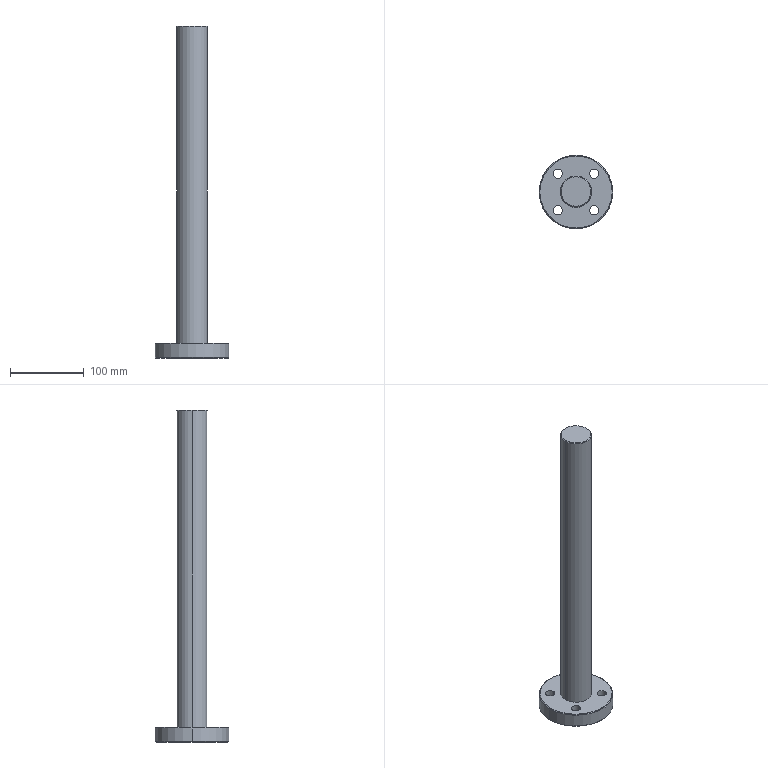Part | SolidWorks | features Chamfer 1, CirPattern 1, Extrusion 1, HoleWzd 1, ICE 1 | 1 solid | 21 faces | box 100 x 100 x 450 mm | volume 742625 mm3 | cylinder 12 | cone 6 | plane 3 | commonest cylinder face diameters 12.5 x8 42 x2 100 x2
STEP:
#1=CARTESIAN_POINT('',(20.,0.,450.));
#2=VERTEX_POINT('',#1);
#3=CARTESIAN_POINT('',(-20.,0.,450.));
#4=VERTEX_POINT('',#3);
#5=CARTESIAN_POINT('',(0.,0.,450.));
#6=DIRECTION('',(0.,0.,1.));
#7=DIRECTION('',(1.,0.,0.));
#8=AXIS2_PLACEMENT_3D('',#5,#6,#7);
#9=CIRCLE('',#8,20.);
#10=EDGE_CURVE('',#2,#4,#9,.T.);
#11=ORIENTED_EDGE('',*,*,#10,.F.);
#12=CARTESIAN_POINT('',(21.,0.,449.));
#13=VERTEX_POINT('',#12);
#14=CARTESIAN_POINT('',(20.,0.,450.));
#15=DIRECTION('',(0.7071,0.,-0.7071));
#16=VECTOR('',#15,1000.);
#17=LINE('',#14,#16);
#18=EDGE_CURVE('',#2,#13,#17,.T.);
#19=ORIENTED_EDGE('',*,*,#18,.T.);
#20=CARTESIAN_POINT('',(-21.,0.,449.));
#21=VERTEX_POINT('',#20);
#22=CARTESIAN_POINT('',(0.,0.,449.));
#23=DIRECTION('',(0.,0.,-1.));
#24=DIRECTION('',(1.,0.,0.));
#25=AXIS2_PLACEMENT_3D('',#22,#23,#24);
#26=CIRCLE('',#25,21.);
#27=EDGE_CURVE('',#21,#13,#26,.T.);
#28=ORIENTED_EDGE('',*,*,#27,.F.);
#29=CARTESIAN_POINT('',(-20.,0.,450.));
#30=DIRECTION('',(-0.7071,0.,-0.7071));
#31=VECTOR('',#30,1000.);
#32=LINE('',#29,#31);
#33=EDGE_CURVE('',#4,#21,#32,.T.);
#34=ORIENTED_EDGE('',*,*,#33,.F.);
#35=EDGE_LOOP('',(#11,#19,#28,#34));
#36=FACE_OUTER_BOUND('',#35,.T.);
#37=CARTESIAN_POINT('',(0.,0.,450.));
#38=DIRECTION('',(0.,0.,-1.));
#39=DIRECTION('',(-1.,0.,0.));
#40=AXIS2_PLACEMENT_3D('',#37,#38,#39);
#41=CONICAL_SURFACE('',#40,20.,0.7854);
#42=ADVANCED_FACE('',(#36),#41,.T.);
#43=CARTESIAN_POINT('',(49.,0.,20.));
#44=VERTEX_POINT('',#43);
#45=CARTESIAN_POINT('',(-49.,0.,20.));
#46=VERTEX_POINT('',#45);
#47=CARTESIAN_POINT('',(0.,0.,20.));
#48=DIRECTION('',(0.,0.,1.));
#49=DIRECTION('',(1.,0.,0.));
#50=AXIS2_PLACEMENT_3D('',#47,#48,#49);
#51=CIRCLE('',#50,49.);
#52=EDGE_CURVE('',#44,#46,#51,.T.);
#53=ORIENTED_EDGE('',*,*,#52,.F.);
#54=CARTESIAN_POINT('',(50.,0.,19.));
#55=VERTEX_POINT('',#54);
#56=CARTESIAN_POINT('',(49.,0.,20.));
#57=DIRECTION('',(0.7071,0.,-0.7071));
#58=VECTOR('',#57,1000.);
#59=LINE('',#56,#58);
#60=EDGE_CURVE('',#44,#55,#59,.T.);
#61=ORIENTED_EDGE('',*,*,#60,.T.);
#62=CARTESIAN_POINT('',(-50.,0.,19.));
#63=VERTEX_POINT('',#62);
#64=CARTESIAN_POINT('',(0.,0.,19.));
#65=DIRECTION('',(0.,0.,-1.));
#66=DIRECTION('',(1.,0.,0.));
#67=AXIS2_PLACEMENT_3D('',#64,#65,#66);
#68=CIRCLE('',#67,50.);
#69=EDGE_CURVE('',#63,#55,#68,.T.);
#70=ORIENTED_EDGE('',*,*,#69,.F.);
#71=CARTESIAN_POINT('',(-49.,0.,20.));
#72=DIRECTION('',(-0.7071,0.,-0.7071));
#73=VECTOR('',#72,1000.);
#74=LINE('',#71,#73);
#75=EDGE_CURVE('',#46,#63,#74,.T.);
#76=ORIENTED_EDGE('',*,*,#75,.F.);
#77=EDGE_LOOP('',(#53,#61,#70,#76));
#78=FACE_OUTER_BOUND('',#77,.T.);
#79=CARTESIAN_POINT('',(0.,0.,20.));
#80=DIRECTION('',(0.,0.,-1.));
#81=DIRECTION('',(-1.,0.,0.));
#82=AXIS2_PLACEMENT_3D('',#79,#80,#81);
#83=CONICAL_SURFACE('',#82,49.,0.7854);
#84=ADVANCED_FACE('',(#78),#83,.T.);
#85=CARTESIAN_POINT('',(-49.,0.,0.));
#86=VERTEX_POINT('',#85);
#87=CARTESIAN_POINT('',(49.,0.,0.));
#88=VERTEX_POINT('',#87);
#89=CARTESIAN_POINT('',(0.,0.,0.));
#90=DIRECTION('',(0.,0.,-1.));
#91=DIRECTION('',(1.,0.,0.));
#92=AXIS2_PLACEMENT_3D('',#89,#90,#91);
#93=CIRCLE('',#92,49.);
#94=EDGE_CURVE('',#86,#88,#93,.T.);
#95=ORIENTED_EDGE('',*,*,#94,.F.);
#96=CARTESIAN_POINT('',(-50.,0.,1.));
#97=VERTEX_POINT('',#96);
#98=CARTESIAN_POINT('',(-50.,0.,1.));
#99=DIRECTION('',(-0.7071,0.,0.7071));
#100=VECTOR('',#99,1000.);
#101=LINE('',#98,#100);
#102=EDGE_CURVE('',#86,#97,#101,.T.);
#103=ORIENTED_EDGE('',*,*,#102,.T.);
#104=CARTESIAN_POINT('',(50.,0.,1.));
#105=VERTEX_POINT('',#104);
#106=CARTESIAN_POINT('',(0.,0.,1.));
#107=DIRECTION('',(0.,0.,1.));
#108=DIRECTION('',(1.,0.,0.));
#109=AXIS2_PLACEMENT_3D('',#106,#107,#108);
#110=CIRCLE('',#109,50.);
#111=EDGE_CURVE('',#105,#97,#110,.T.);
#112=ORIENTED_EDGE('',*,*,#111,.F.);
#113=CARTESIAN_POINT('',(50.,0.,1.));
#114=DIRECTION('',(0.7071,0.,0.7071));
#115=VECTOR('',#114,1000.);
#116=LINE('',#113,#115);
#117=EDGE_CURVE('',#88,#105,#116,.T.);
#118=ORIENTED_EDGE('',*,*,#117,.F.);
#119=EDGE_LOOP('',(#95,#103,#112,#118));
#120=FACE_OUTER_BOUND('',#119,.T.);
#121=CARTESIAN_POINT('',(0.,0.,1.));
#122=DIRECTION('',(0.,0.,1.));
#123=DIRECTION('',(1.,0.,0.));
#124=AXIS2_PLACEMENT_3D('',#121,#122,#123);
#125=CONICAL_SURFACE('',#124,50.,0.7854);
#126=ADVANCED_FACE('',(#120),#125,.T.);
#127=CARTESIAN_POINT('',(18.499,24.749,0.));
#128=VERTEX_POINT('',#127);
#129=CARTESIAN_POINT('',(30.999,24.749,0.));
#130=VERTEX_POINT('',#129);
#131=CARTESIAN_POINT('',(24.749,24.749,0.));
#132=DIRECTION('',(0.,0.,1.));
#133=DIRECTION('',(1.,0.,0.));
#134=AXIS2_PLACEMENT_3D('',#131,#132,#133);
#135=CIRCLE('',#134,6.25);
#136=EDGE_CURVE('',#128,#130,#135,.T.);
#137=ORIENTED_EDGE('',*,*,#136,.F.);
#138=CARTESIAN_POINT('',(18.499,24.749,20.));
#139=VERTEX_POINT('',#138);
#140=CARTESIAN_POINT('',(18.499,24.749,20.));
#141=DIRECTION('',(0.,0.,1.));
#142=VECTOR('',#141,1000.);
#143=LINE('',#140,#142);
#144=EDGE_CURVE('',#128,#139,#143,.T.);
#145=ORIENTED_EDGE('',*,*,#144,.T.);
#146=CARTESIAN_POINT('',(30.999,24.749,20.));
#147=VERTEX_POINT('',#146);
#148=CARTESIAN_POINT('',(24.749,24.749,20.));
#149=DIRECTION('',(0.,0.,1.));
#150=DIRECTION('',(1.,0.,0.));
#151=AXIS2_PLACEMENT_3D('',#148,#149,#150);
#152=CIRCLE('',#151,6.25);
#153=EDGE_CURVE('',#139,#147,#152,.T.);
#154=ORIENTED_EDGE('',*,*,#153,.T.);
#155=CARTESIAN_POINT('',(30.999,24.749,20.));
#156=DIRECTION('',(0.,0.,1.));
#157=VECTOR('',#156,1000.);
#158=LINE('',#155,#157);
#159=EDGE_CURVE('',#130,#147,#158,.T.);
#160=ORIENTED_EDGE('',*,*,#159,.F.);
#161=EDGE_LOOP('',(#137,#145,#154,#160));
#162=FACE_OUTER_BOUND('',#161,.T.);
#163=CARTESIAN_POINT('',(24.749,24.749,20.));
#164=DIRECTION('',(0.,0.,1.));
#165=DIRECTION('',(1.,0.,0.));
#166=AXIS2_PLACEMENT_3D('',#163,#164,#165);
#167=CYLINDRICAL_SURFACE('',#166,6.25);
#168=ADVANCED_FACE('',(#162),#167,.F.);
#169=CARTESIAN_POINT('',(18.499,-24.749,0.));
#170=VERTEX_POINT('',#169);
#171=CARTESIAN_POINT('',(30.999,-24.749,0.));
#172=VERTEX_POINT('',#171);
#173=CARTESIAN_POINT('',(24.749,-24.749,0.));
#174=DIRECTION('',(0.,0.,1.));
#175=DIRECTION('',(1.,0.,0.));
#176=AXIS2_PLACEMENT_3D('',#173,#174,#175);
#177=CIRCLE('',#176,6.25);
#178=EDGE_CURVE('',#170,#172,#177,.T.);
#179=ORIENTED_EDGE('',*,*,#178,.F.);
#180=CARTESIAN_POINT('',(18.499,-24.749,20.));
#181=VERTEX_POINT('',#180);
#182=CARTESIAN_POINT('',(18.499,-24.749,20.));
#183=DIRECTION('',(0.,0.,1.));
#184=VECTOR('',#183,1000.);
#185=LINE('',#182,#184);
#186=EDGE_CURVE('',#170,#181,#185,.T.);
#187=ORIENTED_EDGE('',*,*,#186,.T.);
#188=CARTESIAN_POINT('',(30.999,-24.749,20.));
#189=VERTEX_POINT('',#188);
#190=CARTESIAN_POINT('',(24.749,-24.749,20.));
#191=DIRECTION('',(0.,0.,1.));
#192=DIRECTION('',(1.,0.,0.));
#193=AXIS2_PLACEMENT_3D('',#190,#191,#192);
#194=CIRCLE('',#193,6.25);
#195=EDGE_CURVE('',#181,#189,#194,.T.);
#196=ORIENTED_EDGE('',*,*,#195,.T.);
#197=CARTESIAN_POINT('',(30.999,-24.749,20.));
#198=DIRECTION('',(0.,0.,1.));
#199=VECTOR('',#198,1000.);
#200=LINE('',#197,#199);
#201=EDGE_CURVE('',#172,#189,#200,.T.);
#202=ORIENTED_EDGE('',*,*,#201,.F.);
#203=EDGE_LOOP('',(#179,#187,#196,#202));
#204=FACE_OUTER_BOUND('',#203,.T.);
#205=CARTESIAN_POINT('',(24.749,-24.749,20.));
#206=DIRECTION('',(0.,0.,1.));
#207=DIRECTION('',(1.,0.,0.));
#208=AXIS2_PLACEMENT_3D('',#205,#206,#207);
#209=CYLINDRICAL_SURFACE('',#208,6.25);
#210=ADVANCED_FACE('',(#204),#209,.F.);
#211=CARTESIAN_POINT('',(-30.999,-24.749,0.));
#212=VERTEX_POINT('',#211);
#213=CARTESIAN_POINT('',(-18.499,-24.749,0.));
#214=VERTEX_POINT('',#213);
#215=CARTESIAN_POINT('',(-24.749,-24.749,0.));
#216=DIRECTION('',(0.,0.,1.));
#217=DIRECTION('',(1.,0.,0.));
#218=AXIS2_PLACEMENT_3D('',#215,#216,#217);
#219=CIRCLE('',#218,6.25);
#220=EDGE_CURVE('',#212,#214,#219,.T.);
#221=ORIENTED_EDGE('',*,*,#220,.F.);
#222=CARTESIAN_POINT('',(-30.999,-24.749,20.));
#223=VERTEX_POINT('',#222);
#224=CARTESIAN_POINT('',(-30.999,-24.749,20.));
#225=DIRECTION('',(0.,0.,1.));
#226=VECTOR('',#225,1000.);
#227=LINE('',#224,#226);
#228=EDGE_CURVE('',#212,#223,#227,.T.);
#229=ORIENTED_EDGE('',*,*,#228,.T.);
#230=CARTESIAN_POINT('',(-18.499,-24.749,20.));
#231=VERTEX_POINT('',#230);
#232=CARTESIAN_POINT('',(-24.749,-24.749,20.));
#233=DIRECTION('',(0.,0.,1.));
#234=DIRECTION('',(1.,0.,0.));
#235=AXIS2_PLACEMENT_3D('',#232,#233,#234);
#236=CIRCLE('',#235,6.25);
#237=EDGE_CURVE('',#223,#231,#236,.T.);
#238=ORIENTED_EDGE('',*,*,#237,.T.);
#239=CARTESIAN_POINT('',(-18.499,-24.749,20.));
#240=DIRECTION('',(0.,0.,1.));
#241=VECTOR('',#240,1000.);
#242=LINE('',#239,#241);
#243=EDGE_CURVE('',#214,#231,#242,.T.);
#244=ORIENTED_EDGE('',*,*,#243,.F.);
#245=EDGE_LOOP('',(#221,#229,#238,#244));
#246=FACE_OUTER_BOUND('',#245,.T.);
#247=CARTESIAN_POINT('',(-24.749,-24.749,20.));
#248=DIRECTION('',(0.,0.,1.));
#249=DIRECTION('',(1.,0.,0.));
#250=AXIS2_PLACEMENT_3D('',#247,#248,#249);
#251=CYLINDRICAL_SURFACE('',#250,6.25);
#252=ADVANCED_FACE('',(#246),#251,.F.);
#253=CARTESIAN_POINT('',(-30.999,24.749,0.));
#254=VERTEX_POINT('',#253);
#255=CARTESIAN_POINT('',(-18.499,24.749,0.));
#256=VERTEX_POINT('',#255);
#257=CARTESIAN_POINT('',(-24.749,24.749,0.));
#258=DIRECTION('',(0.,0.,1.));
#259=DIRECTION('',(1.,0.,0.));
#260=AXIS2_PLACEMENT_3D('',#257,#258,#259);
#261=CIRCLE('',#260,6.25);
#262=EDGE_CURVE('',#254,#256,#261,.T.);
#263=ORIENTED_EDGE('',*,*,#262,.F.);
#264=CARTESIAN_POINT('',(-30.999,24.749,20.));
#265=VERTEX_POINT('',#264);
#266=CARTESIAN_POINT('',(-30.999,24.749,20.));
#267=DIRECTION('',(0.,0.,1.));
#268=VECTOR('',#267,1000.);
#269=LINE('',#266,#268);
#270=EDGE_CURVE('',#254,#265,#269,.T.);
#271=ORIENTED_EDGE('',*,*,#270,.T.);
#272=CARTESIAN_POINT('',(-18.499,24.749,20.));
#273=VERTEX_POINT('',#272);
#274=CARTESIAN_POINT('',(-24.749,24.749,20.));
#275=DIRECTION('',(0.,0.,1.));
#276=DIRECTION('',(1.,0.,0.));
#277=AXIS2_PLACEMENT_3D('',#274,#275,#276);
#278=CIRCLE('',#277,6.25);
#279=EDGE_CURVE('',#265,#273,#278,.T.);
#280=ORIENTED_EDGE('',*,*,#279,.T.);
#281=CARTESIAN_POINT('',(-18.499,24.749,20.));
#282=DIRECTION('',(0.,0.,1.));
#283=VECTOR('',#282,1000.);
#284=LINE('',#281,#283);
#285=EDGE_CURVE('',#256,#273,#284,.T.);
#286=ORIENTED_EDGE('',*,*,#285,.F.);
#287=EDGE_LOOP('',(#263,#271,#280,#286));
#288=FACE_OUTER_BOUND('',#287,.T.);
#289=CARTESIAN_POINT('',(-24.749,24.749,20.));
#290=DIRECTION('',(0.,0.,1.));
#291=DIRECTION('',(1.,0.,0.));
#292=AXIS2_PLACEMENT_3D('',#289,#290,#291);
#293=CYLINDRICAL_SURFACE('',#292,6.25);
#294=ADVANCED_FACE('',(#288),#293,.F.);
#295=ORIENTED_EDGE('',*,*,#27,.T.);
#296=CARTESIAN_POINT('',(21.,0.,20.));
#297=VERTEX_POINT('',#296);
#298=CARTESIAN_POINT('',(21.,0.,450.));
#299=DIRECTION('',(0.,0.,-1.));
#300=VECTOR('',#299,1000.);
#301=LINE('',#298,#300);
#302=EDGE_CURVE('',#13,#297,#301,.T.);
#303=ORIENTED_EDGE('',*,*,#302,.T.);
#304=CARTESIAN_POINT('',(-21.,0.,20.));
#305=VERTEX_POINT('',#304);
#306=CARTESIAN_POINT('',(0.,0.,20.));
#307=DIRECTION('',(0.,0.,1.));
#308=DIRECTION('',(1.,0.,0.));
#309=AXIS2_PLACEMENT_3D('',#306,#307,#308);
#310=CIRCLE('',#309,21.);
#311=EDGE_CURVE('',#297,#305,#310,.T.);
#312=ORIENTED_EDGE('',*,*,#311,.T.);
#313=CARTESIAN_POINT('',(-21.,0.,450.));
#314=DIRECTION('',(0.,0.,-1.));
#315=VECTOR('',#314,1000.);
#316=LINE('',#313,#315);
#317=EDGE_CURVE('',#21,#305,#316,.T.);
#318=ORIENTED_EDGE('',*,*,#317,.F.);
#319=EDGE_LOOP('',(#295,#303,#312,#318));
#320=FACE_OUTER_BOUND('',#319,.T.);
#321=CARTESIAN_POINT('',(0.,0.,450.));
#322=DIRECTION('',(0.,0.,-1.));
#323=DIRECTION('',(-1.,0.,0.));
#324=AXIS2_PLACEMENT_3D('',#321,#322,#323);
#325=CYLINDRICAL_SURFACE('',#324,21.);
#326=ADVANCED_FACE('',(#320),#325,.T.);
#327=ORIENTED_EDGE('',*,*,#69,.T.);
#328=CARTESIAN_POINT('',(50.,0.,20.));
#329=DIRECTION('',(0.,0.,-1.));
#330=VECTOR('',#329,1000.);
#331=LINE('',#328,#330);
#332=EDGE_CURVE('',#55,#105,#331,.T.);
#333=ORIENTED_EDGE('',*,*,#332,.T.);
#334=ORIENTED_EDGE('',*,*,#111,.T.);
#335=CARTESIAN_POINT('',(-50.,0.,20.));
#336=DIRECTION('',(0.,0.,-1.));
#337=VECTOR('',#336,1000.);
#338=LINE('',#335,#337);
#339=EDGE_CURVE('',#63,#97,#338,.T.);
#340=ORIENTED_EDGE('',*,*,#339,.F.);
#341=EDGE_LOOP('',(#327,#333,#334,#340));
#342=FACE_OUTER_BOUND('',#341,.T.);
#343=CARTESIAN_POINT('',(0.,0.,20.));
#344=DIRECTION('',(0.,0.,-1.));
#345=DIRECTION('',(-1.,0.,0.));
#346=AXIS2_PLACEMENT_3D('',#343,#344,#345);
#347=CYLINDRICAL_SURFACE('',#346,50.);
#348=ADVANCED_FACE('',(#342),#347,.T.);
#349=ORIENTED_EDGE('',*,*,#332,.F.);
#350=CARTESIAN_POINT('',(0.,0.,19.));
#351=DIRECTION('',(0.,0.,-1.));
#352=DIRECTION('',(1.,0.,0.));
#353=AXIS2_PLACEMENT_3D('',#350,#351,#352);
#354=CIRCLE('',#353,50.);
#355=EDGE_CURVE('',#55,#63,#354,.T.);
#356=ORIENTED_EDGE('',*,*,#355,.T.);
#357=ORIENTED_EDGE('',*,*,#339,.T.);
#358=CARTESIAN_POINT('',(0.,0.,1.));
#359=DIRECTION('',(0.,0.,1.));
#360=DIRECTION('',(1.,0.,0.));
#361=AXIS2_PLACEMENT_3D('',#358,#359,#360);
#362=CIRCLE('',#361,50.);
#363=EDGE_CURVE('',#97,#105,#362,.T.);
#364=ORIENTED_EDGE('',*,*,#363,.T.);
#365=EDGE_LOOP('',(#349,#356,#357,#364));
#366=FACE_OUTER_BOUND('',#365,.T.);
#367=CARTESIAN_POINT('',(0.,0.,20.));
#368=DIRECTION('',(0.,0.,-1.));
#369=DIRECTION('',(-1.,0.,0.));
#370=AXIS2_PLACEMENT_3D('',#367,#368,#369);
#371=CYLINDRICAL_SURFACE('',#370,50.);
#372=ADVANCED_FACE('',(#366),#371,.T.);
#373=CARTESIAN_POINT('',(0.,0.,20.));
#374=DIRECTION('',(0.,0.,1.));
#375=DIRECTION('',(1.,0.,0.));
#376=AXIS2_PLACEMENT_3D('',#373,#374,#375);
#377=CIRCLE('',#376,49.);
#378=EDGE_CURVE('',#46,#44,#377,.T.);
#379=ORIENTED_EDGE('',*,*,#378,.T.);
#380=ORIENTED_EDGE('',*,*,#52,.T.);
#381=EDGE_LOOP('',(#379,#380));
#382=FACE_OUTER_BOUND('',#381,.T.);
#383=CARTESIAN_POINT('',(24.749,24.749,20.));
#384=DIRECTION('',(0.,0.,1.));
#385=DIRECTION('',(1.,0.,0.));
#386=AXIS2_PLACEMENT_3D('',#383,#384,#385);
#387=CIRCLE('',#386,6.25);
#388=EDGE_CURVE('',#147,#139,#387,.T.);
#389=ORIENTED_EDGE('',*,*,#388,.F.);
#390=ORIENTED_EDGE('',*,*,#153,.F.);
#391=EDGE_LOOP('',(#389,#390));
#392=FACE_BOUND('',#391,.T.);
#393=CARTESIAN_POINT('',(24.749,-24.749,20.));
#394=DIRECTION('',(0.,0.,1.));
#395=DIRECTION('',(1.,0.,0.));
#396=AXIS2_PLACEMENT_3D('',#393,#394,#395);
#397=CIRCLE('',#396,6.25);
#398=EDGE_CURVE('',#189,#181,#397,.T.);
#399=ORIENTED_EDGE('',*,*,#398,.F.);
#400=ORIENTED_EDGE('',*,*,#195,.F.);
#401=EDGE_LOOP('',(#399,#400));
#402=FACE_BOUND('',#401,.T.);
#403=CARTESIAN_POINT('',(-24.749,-24.749,20.));
#404=DIRECTION('',(0.,0.,1.));
#405=DIRECTION('',(1.,0.,0.));
#406=AXIS2_PLACEMENT_3D('',#403,#404,#405);
#407=CIRCLE('',#406,6.25);
#408=EDGE_CURVE('',#231,#223,#407,.T.);
#409=ORIENTED_EDGE('',*,*,#408,.F.);
#410=ORIENTED_EDGE('',*,*,#237,.F.);
#411=EDGE_LOOP('',(#409,#410));
#412=FACE_BOUND('',#411,.T.);
#413=CARTESIAN_POINT('',(-24.749,24.749,20.));
#414=DIRECTION('',(0.,0.,1.));
#415=DIRECTION('',(1.,0.,0.));
#416=AXIS2_PLACEMENT_3D('',#413,#414,#415);
#417=CIRCLE('',#416,6.25);
#418=EDGE_CURVE('',#273,#265,#417,.T.);
#419=ORIENTED_EDGE('',*,*,#418,.F.);
#420=ORIENTED_EDGE('',*,*,#279,.F.);
#421=EDGE_LOOP('',(#419,#420));
#422=FACE_BOUND('',#421,.T.);
#423=CARTESIAN_POINT('',(0.,0.,20.));
#424=DIRECTION('',(0.,0.,1.));
#425=DIRECTION('',(1.,0.,0.));
#426=AXIS2_PLACEMENT_3D('',#423,#424,#425);
#427=CIRCLE('',#426,21.);
#428=EDGE_CURVE('',#305,#297,#427,.T.);
#429=ORIENTED_EDGE('',*,*,#428,.F.);
#430=ORIENTED_EDGE('',*,*,#311,.F.);
#431=EDGE_LOOP('',(#429,#430));
#432=FACE_BOUND('',#431,.T.);
#433=CARTESIAN_POINT('',(0.,0.,20.));
#434=DIRECTION('',(0.,0.,1.));
#435=DIRECTION('',(1.,0.,0.));
#436=AXIS2_PLACEMENT_3D('',#433,#434,#435);
#437=PLANE('',#436);
#438=ADVANCED_FACE('',(#382,#392,#402,#412,#422,#432),#437,.T.);
#439=CARTESIAN_POINT('',(0.,0.,0.));
#440=DIRECTION('',(0.,0.,-1.));
#441=DIRECTION('',(1.,0.,0.));
#442=AXIS2_PLACEMENT_3D('',#439,#440,#441);
#443=CIRCLE('',#442,49.);
#444=EDGE_CURVE('',#88,#86,#443,.T.);
#445=ORIENTED_EDGE('',*,*,#444,.T.);
#446=ORIENTED_EDGE('',*,*,#94,.T.);
#447=EDGE_LOOP('',(#445,#446));
#448=FACE_OUTER_BOUND('',#447,.T.);
#449=CARTESIAN_POINT('',(24.749,24.749,0.));
#450=DIRECTION('',(0.,0.,1.));
#451=DIRECTION('',(1.,0.,0.));
#452=AXIS2_PLACEMENT_3D('',#449,#450,#451);
#453=CIRCLE('',#452,6.25);
#454=EDGE_CURVE('',#130,#128,#453,.T.);
#455=ORIENTED_EDGE('',*,*,#454,.T.);
#456=ORIENTED_EDGE('',*,*,#136,.T.);
#457=EDGE_LOOP('',(#455,#456));
#458=FACE_BOUND('',#457,.T.);
#459=CARTESIAN_POINT('',(24.749,-24.749,0.));
#460=DIRECTION('',(0.,0.,1.));
#461=DIRECTION('',(1.,0.,0.));
#462=AXIS2_PLACEMENT_3D('',#459,#460,#461);
#463=CIRCLE('',#462,6.25);
#464=EDGE_CURVE('',#172,#170,#463,.T.);
#465=ORIENTED_EDGE('',*,*,#464,.T.);
#466=ORIENTED_EDGE('',*,*,#178,.T.);
#467=EDGE_LOOP('',(#465,#466));
#468=FACE_BOUND('',#467,.T.);
#469=CARTESIAN_POINT('',(-24.749,-24.749,0.));
#470=DIRECTION('',(0.,0.,1.));
#471=DIRECTION('',(1.,0.,0.));
#472=AXIS2_PLACEMENT_3D('',#469,#470,#471);
#473=CIRCLE('',#472,6.25);
#474=EDGE_CURVE('',#214,#212,#473,.T.);
#475=ORIENTED_EDGE('',*,*,#474,.T.);
#476=ORIENTED_EDGE('',*,*,#220,.T.);
#477=EDGE_LOOP('',(#475,#476));
#478=FACE_BOUND('',#477,.T.);
#479=CARTESIAN_POINT('',(-24.749,24.749,0.));
#480=DIRECTION('',(0.,0.,1.));
#481=DIRECTION('',(1.,0.,0.));
#482=AXIS2_PLACEMENT_3D('',#479,#480,#481);
#483=CIRCLE('',#482,6.25);
#484=EDGE_CURVE('',#256,#254,#483,.T.);
#485=ORIENTED_EDGE('',*,*,#484,.T.);
#486=ORIENTED_EDGE('',*,*,#262,.T.);
#487=EDGE_LOOP('',(#485,#486));
#488=FACE_BOUND('',#487,.T.);
#489=CARTESIAN_POINT('',(0.,0.,0.));
#490=DIRECTION('',(0.,0.,1.));
#491=DIRECTION('',(1.,0.,0.));
#492=AXIS2_PLACEMENT_3D('',#489,#490,#491);
#493=PLANE('',#492);
#494=ADVANCED_FACE('',(#448,#458,#468,#478,#488),#493,.F.);
#495=ORIENTED_EDGE('',*,*,#302,.F.);
#496=CARTESIAN_POINT('',(0.,0.,449.));
#497=DIRECTION('',(0.,0.,-1.));
#498=DIRECTION('',(1.,0.,0.));
#499=AXIS2_PLACEMENT_3D('',#496,#497,#498);
#500=CIRCLE('',#499,21.);
#501=EDGE_CURVE('',#13,#21,#500,.T.);
#502=ORIENTED_EDGE('',*,*,#501,.T.);
#503=ORIENTED_EDGE('',*,*,#317,.T.);
#504=ORIENTED_EDGE('',*,*,#428,.T.);
#505=EDGE_LOOP('',(#495,#502,#503,#504));
#506=FACE_OUTER_BOUND('',#505,.T.);
#507=CARTESIAN_POINT('',(0.,0.,450.));
#508=DIRECTION('',(0.,0.,-1.));
#509=DIRECTION('',(-1.,0.,0.));
#510=AXIS2_PLACEMENT_3D('',#507,#508,#509);
#511=CYLINDRICAL_SURFACE('',#510,21.);
#512=ADVANCED_FACE('',(#506),#511,.T.);
#513=CARTESIAN_POINT('',(0.,0.,450.));
#514=DIRECTION('',(0.,0.,1.));
#515=DIRECTION('',(1.,0.,0.));
#516=AXIS2_PLACEMENT_3D('',#513,#514,#515);
#517=CIRCLE('',#516,20.);
#518=EDGE_CURVE('',#4,#2,#517,.T.);
#519=ORIENTED_EDGE('',*,*,#518,.T.);
#520=ORIENTED_EDGE('',*,*,#10,.T.);
#521=EDGE_LOOP('',(#519,#520));
#522=FACE_OUTER_BOUND('',#521,.T.);
#523=CARTESIAN_POINT('',(0.,0.,450.));
#524=DIRECTION('',(0.,0.,1.));
#525=DIRECTION('',(1.,0.,0.));
#526=AXIS2_PLACEMENT_3D('',#523,#524,#525);
#527=PLANE('',#526);
#528=ADVANCED_FACE('',(#522),#527,.T.);
#529=ORIENTED_EDGE('',*,*,#270,.F.);
#530=ORIENTED_EDGE('',*,*,#484,.F.);
#531=ORIENTED_EDGE('',*,*,#285,.T.);
#532=ORIENTED_EDGE('',*,*,#418,.T.);
#533=EDGE_LOOP('',(#529,#530,#531,#532));
#534=FACE_OUTER_BOUND('',#533,.T.);
#535=CARTESIAN_POINT('',(-24.749,24.749,20.));
#536=DIRECTION('',(0.,0.,1.));
#537=DIRECTION('',(1.,0.,0.));
#538=AXIS2_PLACEMENT_3D('',#535,#536,#537);
#539=CYLINDRICAL_SURFACE('',#538,6.25);
#540=ADVANCED_FACE('',(#534),#539,.F.);
#541=ORIENTED_EDGE('',*,*,#228,.F.);
#542=ORIENTED_EDGE('',*,*,#474,.F.);
#543=ORIENTED_EDGE('',*,*,#243,.T.);
#544=ORIENTED_EDGE('',*,*,#408,.T.);
#545=EDGE_LOOP('',(#541,#542,#543,#544));
#546=FACE_OUTER_BOUND('',#545,.T.);
#547=CARTESIAN_POINT('',(-24.749,-24.749,20.));
#548=DIRECTION('',(0.,0.,1.));
#549=DIRECTION('',(1.,0.,0.));
#550=AXIS2_PLACEMENT_3D('',#547,#548,#549);
#551=CYLINDRICAL_SURFACE('',#550,6.25);
#552=ADVANCED_FACE('',(#546),#551,.F.);
#553=ORIENTED_EDGE('',*,*,#186,.F.);
#554=ORIENTED_EDGE('',*,*,#464,.F.);
#555=ORIENTED_EDGE('',*,*,#201,.T.);
#556=ORIENTED_EDGE('',*,*,#398,.T.);
#557=EDGE_LOOP('',(#553,#554,#555,#556));
#558=FACE_OUTER_BOUND('',#557,.T.);
#559=CARTESIAN_POINT('',(24.749,-24.749,20.));
#560=DIRECTION('',(0.,0.,1.));
#561=DIRECTION('',(1.,0.,0.));
#562=AXIS2_PLACEMENT_3D('',#559,#560,#561);
#563=CYLINDRICAL_SURFACE('',#562,6.25);
#564=ADVANCED_FACE('',(#558),#563,.F.);
#565=ORIENTED_EDGE('',*,*,#144,.F.);
#566=ORIENTED_EDGE('',*,*,#454,.F.);
#567=ORIENTED_EDGE('',*,*,#159,.T.);
#568=ORIENTED_EDGE('',*,*,#388,.T.);
#569=EDGE_LOOP('',(#565,#566,#567,#568));
#570=FACE_OUTER_BOUND('',#569,.T.);
#571=CARTESIAN_POINT('',(24.749,24.749,20.));
#572=DIRECTION('',(0.,0.,1.));
#573=DIRECTION('',(1.,0.,0.));
#574=AXIS2_PLACEMENT_3D('',#571,#572,#573);
#575=CYLINDRICAL_SURFACE('',#574,6.25);
#576=ADVANCED_FACE('',(#570),#575,.F.);
#577=ORIENTED_EDGE('',*,*,#102,.F.);
#578=ORIENTED_EDGE('',*,*,#444,.F.);
#579=ORIENTED_EDGE('',*,*,#117,.T.);
#580=ORIENTED_EDGE('',*,*,#363,.F.);
#581=EDGE_LOOP('',(#577,#578,#579,#580));
#582=FACE_OUTER_BOUND('',#581,.T.);
#583=CARTESIAN_POINT('',(0.,0.,1.));
#584=DIRECTION('',(0.,0.,1.));
#585=DIRECTION('',(1.,0.,0.));
#586=AXIS2_PLACEMENT_3D('',#583,#584,#585);
#587=CONICAL_SURFACE('',#586,50.,0.7854);
#588=ADVANCED_FACE('',(#582),#587,.T.);
#589=ORIENTED_EDGE('',*,*,#60,.F.);
#590=ORIENTED_EDGE('',*,*,#378,.F.);
#591=ORIENTED_EDGE('',*,*,#75,.T.);
#592=ORIENTED_EDGE('',*,*,#355,.F.);
#593=EDGE_LOOP('',(#589,#590,#591,#592));
#594=FACE_OUTER_BOUND('',#593,.T.);
#595=CARTESIAN_POINT('',(0.,0.,20.));
#596=DIRECTION('',(0.,0.,-1.));
#597=DIRECTION('',(-1.,0.,0.));
#598=AXIS2_PLACEMENT_3D('',#595,#596,#597);
#599=CONICAL_SURFACE('',#598,49.,0.7854);
#600=ADVANCED_FACE('',(#594),#599,.T.);
#601=ORIENTED_EDGE('',*,*,#18,.F.);
#602=ORIENTED_EDGE('',*,*,#518,.F.);
#603=ORIENTED_EDGE('',*,*,#33,.T.);
#604=ORIENTED_EDGE('',*,*,#501,.F.);
#605=EDGE_LOOP('',(#601,#602,#603,#604));
#606=FACE_OUTER_BOUND('',#605,.T.);
#607=CARTESIAN_POINT('',(0.,0.,450.));
#608=DIRECTION('',(0.,0.,-1.));
#609=DIRECTION('',(-1.,0.,0.));
#610=AXIS2_PLACEMENT_3D('',#607,#608,#609);
#611=CONICAL_SURFACE('',#610,20.,0.7854);
#612=ADVANCED_FACE('',(#606),#611,.T.);
#613=CLOSED_SHELL('',(#42,#84,#126,#168,#210,#252,#294,#326,#348,#372,#438,#494,#512,#528,#540,#552,#564,#576,#588,#600,#612));
#614=MANIFOLD_SOLID_BREP('',#613);
#615=CARTESIAN_POINT('',(0.,0.,0.));
#616=DIRECTION('',(0.,0.,1.));
#617=DIRECTION('',(1.,0.,0.));
#618=AXIS2_PLACEMENT_3D('',#615,#616,#617);
#619=(LENGTH_UNIT()NAMED_UNIT(*)SI_UNIT(.MILLI.,.METRE.));
#620=UNCERTAINTY_MEASURE_WITH_UNIT(LENGTH_MEASURE(0.00001),#619,'','');
#621=(NAMED_UNIT(*)PLANE_ANGLE_UNIT()SI_UNIT($,.RADIAN.));
#622=(NAMED_UNIT(*)SI_UNIT($,.STERADIAN.)SOLID_ANGLE_UNIT());
#623=(GEOMETRIC_REPRESENTATION_CONTEXT(3)GLOBAL_UNCERTAINTY_ASSIGNED_CONTEXT((#620))GLOBAL_UNIT_ASSIGNED_CONTEXT((#619,#621,#622))REPRESENTATION_CONTEXT('',''));
#624=ADVANCED_BREP_SHAPE_REPRESENTATION('',(#614,#618),#623);